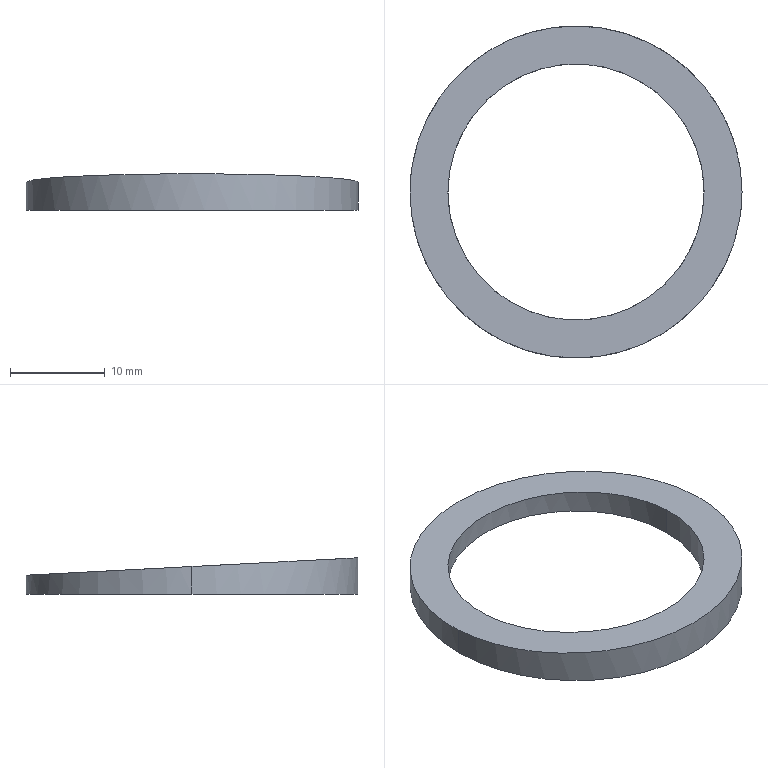Part | STEP file | TCHK-2D-D30-BB-5.stp.STEP | 1 solid | 6 faces | box 35 x 35 x 3.834 mm | volume 1137 mm3 | cylinder 4 | plane 2 | commonest cylinder face diameters 27 x2 35 x2
STEP:
#1=CARTESIAN_POINT('',(13.5,0.,0.));
#2=VERTEX_POINT('',#1);
#3=CARTESIAN_POINT('',(-13.5,0.,0.));
#4=VERTEX_POINT('',#3);
#5=CARTESIAN_POINT('',(0.,0.,0.));
#6=DIRECTION('',(0.,0.,-1.));
#7=DIRECTION('',(1.,0.,0.));
#8=AXIS2_PLACEMENT_3D('',#5,#6,#7);
#9=CIRCLE('',#8,13.5);
#10=EDGE_CURVE('',#2,#4,#9,.T.);
#11=ORIENTED_EDGE('',*,*,#10,.F.);
#12=CARTESIAN_POINT('',(0.,0.,0.));
#13=DIRECTION('',(0.,0.,-1.));
#14=DIRECTION('',(-1.,0.,0.));
#15=AXIS2_PLACEMENT_3D('',#12,#13,#14);
#16=CIRCLE('',#15,13.5);
#17=EDGE_CURVE('',#4,#2,#16,.T.);
#18=ORIENTED_EDGE('',*,*,#17,.F.);
#19=EDGE_LOOP('',(#11,#18));
#20=FACE_BOUND('',#19,.T.);
#21=CARTESIAN_POINT('',(-17.5,0.,0.));
#22=VERTEX_POINT('',#21);
#23=CARTESIAN_POINT('',(17.5,0.,0.));
#24=VERTEX_POINT('',#23);
#25=CARTESIAN_POINT('',(0.,0.,0.));
#26=DIRECTION('',(0.,0.,1.));
#27=DIRECTION('',(-1.,0.,0.));
#28=AXIS2_PLACEMENT_3D('',#25,#26,#27);
#29=CIRCLE('',#28,17.5);
#30=EDGE_CURVE('',#22,#24,#29,.T.);
#31=ORIENTED_EDGE('',*,*,#30,.F.);
#32=CARTESIAN_POINT('',(0.,0.,0.));
#33=DIRECTION('',(0.,0.,1.));
#34=DIRECTION('',(1.,0.,0.));
#35=AXIS2_PLACEMENT_3D('',#32,#33,#34);
#36=CIRCLE('',#35,17.5);
#37=EDGE_CURVE('',#24,#22,#36,.T.);
#38=ORIENTED_EDGE('',*,*,#37,.F.);
#39=EDGE_LOOP('',(#31,#38));
#40=FACE_OUTER_BOUND('',#39,.T.);
#41=CARTESIAN_POINT('',(0.,0.,0.));
#42=DIRECTION('',(0.,0.,1.));
#43=DIRECTION('',(1.,0.,0.));
#44=AXIS2_PLACEMENT_3D('',#41,#42,#43);
#45=PLANE('',#44);
#46=ADVANCED_FACE('',(#20,#40),#45,.F.);
#47=CARTESIAN_POINT('',(17.5,0.,2.917));
#48=VERTEX_POINT('',#47);
#49=CARTESIAN_POINT('',(17.5,0.,0.));
#50=DIRECTION('',(0.,0.,1.));
#51=VECTOR('',#50,1000.);
#52=LINE('',#49,#51);
#53=EDGE_CURVE('',#24,#48,#52,.T.);
#54=ORIENTED_EDGE('',*,*,#53,.F.);
#55=ORIENTED_EDGE('',*,*,#37,.T.);
#56=CARTESIAN_POINT('',(-17.5,0.,2.917));
#57=VERTEX_POINT('',#56);
#58=CARTESIAN_POINT('',(-17.5,0.,0.));
#59=DIRECTION('',(0.,0.,1.));
#60=VECTOR('',#59,1000.);
#61=LINE('',#58,#60);
#62=EDGE_CURVE('',#22,#57,#61,.T.);
#63=ORIENTED_EDGE('',*,*,#62,.T.);
#64=CARTESIAN_POINT('',(17.5,0.,2.917));
#65=CARTESIAN_POINT('',(17.5,0.5353,2.889));
#66=CARTESIAN_POINT('',(17.463,1.335,2.847));
#67=CARTESIAN_POINT('',(17.357,2.262,2.799));
#68=CARTESIAN_POINT('',(17.288,2.723,2.774));
#69=CARTESIAN_POINT('',(17.249,2.954,2.762));
#70=CARTESIAN_POINT('',(17.232,3.053,2.757));
#71=CARTESIAN_POINT('',(17.22,3.119,2.754));
#72=CARTESIAN_POINT('',(17.214,3.149,2.752));
#73=CARTESIAN_POINT('',(17.105,3.742,2.721));
#74=CARTESIAN_POINT('',(16.91,4.568,2.678));
#75=CARTESIAN_POINT('',(16.614,5.512,2.628));
#76=CARTESIAN_POINT('',(16.448,5.978,2.604));
#77=CARTESIAN_POINT('',(16.361,6.21,2.592));
#78=CARTESIAN_POINT('',(16.323,6.31,2.586));
#79=CARTESIAN_POINT('',(16.297,6.376,2.583));
#80=CARTESIAN_POINT('',(16.285,6.407,2.581));
#81=CARTESIAN_POINT('',(16.054,6.991,2.551));
#82=CARTESIAN_POINT('',(15.687,7.796,2.509));
#83=CARTESIAN_POINT('',(15.191,8.698,2.461));
#84=CARTESIAN_POINT('',(14.925,9.14,2.438));
#85=CARTESIAN_POINT('',(14.807,9.328,2.428));
#86=CARTESIAN_POINT('',(14.728,9.452,2.422));
#87=CARTESIAN_POINT('',(14.689,9.513,2.419));
#88=CARTESIAN_POINT('',(13.987,10.587,2.362));
#89=CARTESIAN_POINT('',(13.228,11.521,2.313));
#90=CARTESIAN_POINT('',(11.948,12.801,2.246));
#91=CARTESIAN_POINT('',(11.278,13.406,2.215));
#92=CARTESIAN_POINT('',(10.444,14.047,2.181));
#93=CARTESIAN_POINT('',(10.015,14.353,2.165));
#94=CARTESIAN_POINT('',(9.828,14.48,2.158));
#95=CARTESIAN_POINT('',(9.702,14.564,2.154));
#96=CARTESIAN_POINT('',(9.638,14.607,2.152));
#97=CARTESIAN_POINT('',(9.082,14.971,2.133));
#98=CARTESIAN_POINT('',(8.319,15.416,2.109));
#99=CARTESIAN_POINT('',(7.393,15.867,2.086));
#100=CARTESIAN_POINT('',(6.92,16.075,2.075));
#101=CARTESIAN_POINT('',(6.682,16.174,2.069));
#102=CARTESIAN_POINT('',(6.579,16.216,2.067));
#103=CARTESIAN_POINT('',(6.51,16.244,2.066));
#104=CARTESIAN_POINT('',(6.475,16.258,2.065));
#105=CARTESIAN_POINT('',(5.915,16.48,2.053));
#106=CARTESIAN_POINT('',(5.113,16.754,2.039));
#107=CARTESIAN_POINT('',(4.155,17.004,2.026));
#108=CARTESIAN_POINT('',(3.672,17.112,2.02));
#109=CARTESIAN_POINT('',(3.428,17.161,2.018));
#110=CARTESIAN_POINT('',(3.324,17.181,2.017));
#111=CARTESIAN_POINT('',(3.254,17.195,2.016));
#112=CARTESIAN_POINT('',(3.217,17.202,2.016));
#113=CARTESIAN_POINT('',(2.133,17.403,2.005));
#114=CARTESIAN_POINT('',(1.07,17.5,2.));
#115=CARTESIAN_POINT('',(-0.535,17.5,2.));
#116=CARTESIAN_POINT('',(-1.334,17.464,2.002));
#117=CARTESIAN_POINT('',(-2.261,17.357,2.007));
#118=CARTESIAN_POINT('',(-2.723,17.288,2.011));
#119=CARTESIAN_POINT('',(-2.954,17.249,2.013));
#120=CARTESIAN_POINT('',(-3.053,17.232,2.014));
#121=CARTESIAN_POINT('',(-3.119,17.22,2.015));
#122=CARTESIAN_POINT('',(-3.149,17.214,2.015));
#123=CARTESIAN_POINT('',(-3.743,17.105,2.021));
#124=CARTESIAN_POINT('',(-4.569,16.91,2.031));
#125=CARTESIAN_POINT('',(-5.512,16.614,2.046));
#126=CARTESIAN_POINT('',(-5.978,16.448,2.055));
#127=CARTESIAN_POINT('',(-6.21,16.361,2.06));
#128=CARTESIAN_POINT('',(-6.31,16.323,2.062));
#129=CARTESIAN_POINT('',(-6.376,16.297,2.063));
#130=CARTESIAN_POINT('',(-6.407,16.285,2.064));
#131=CARTESIAN_POINT('',(-6.992,16.054,2.076));
#132=CARTESIAN_POINT('',(-7.796,15.687,2.095));
#133=CARTESIAN_POINT('',(-8.698,15.19,2.121));
#134=CARTESIAN_POINT('',(-9.14,14.925,2.135));
#135=CARTESIAN_POINT('',(-9.328,14.807,2.141));
#136=CARTESIAN_POINT('',(-9.452,14.728,2.145));
#137=CARTESIAN_POINT('',(-9.513,14.689,2.147));
#138=CARTESIAN_POINT('',(-10.587,13.987,2.184));
#139=CARTESIAN_POINT('',(-11.521,13.228,2.224));
#140=CARTESIAN_POINT('',(-12.801,11.948,2.291));
#141=CARTESIAN_POINT('',(-13.405,11.278,2.326));
#142=CARTESIAN_POINT('',(-14.047,10.444,2.37));
#143=CARTESIAN_POINT('',(-14.353,10.015,2.392));
#144=CARTESIAN_POINT('',(-14.48,9.828,2.402));
#145=CARTESIAN_POINT('',(-14.564,9.702,2.409));
#146=CARTESIAN_POINT('',(-14.607,9.638,2.412));
#147=CARTESIAN_POINT('',(-14.971,9.082,2.441));
#148=CARTESIAN_POINT('',(-15.416,8.319,2.481));
#149=CARTESIAN_POINT('',(-15.867,7.393,2.53));
#150=CARTESIAN_POINT('',(-16.075,6.92,2.554));
#151=CARTESIAN_POINT('',(-16.174,6.682,2.567));
#152=CARTESIAN_POINT('',(-16.216,6.579,2.572));
#153=CARTESIAN_POINT('',(-16.244,6.51,2.576));
#154=CARTESIAN_POINT('',(-16.258,6.475,2.578));
#155=CARTESIAN_POINT('',(-16.48,5.915,2.607));
#156=CARTESIAN_POINT('',(-16.754,5.112,2.649));
#157=CARTESIAN_POINT('',(-17.004,4.155,2.699));
#158=CARTESIAN_POINT('',(-17.112,3.672,2.725));
#159=CARTESIAN_POINT('',(-17.161,3.428,2.737));
#160=CARTESIAN_POINT('',(-17.181,3.324,2.743));
#161=CARTESIAN_POINT('',(-17.195,3.254,2.747));
#162=CARTESIAN_POINT('',(-17.202,3.217,2.749));
#163=CARTESIAN_POINT('',(-17.403,2.133,2.805));
#164=CARTESIAN_POINT('',(-17.5,1.071,2.861));
#165=CARTESIAN_POINT('',(-17.5,0.,2.917));
#166=B_SPLINE_CURVE_WITH_KNOTS('',3,(#64,#65,#66,#67,#68,#69,#70,#71,#72,#73,#74,#75,#76,#77,#78,#79,#80,#81,#82,#83,#84,#85,#86,#87,#88,#89,#90,#91,#92,#93,#94,#95,#96,#97,#98,#99,#100,#101,#102,#103,#104,#105,#106,#107,#108,#109,#110,#111,#112,#113,#114,#115,#116,#117,#118,#119,#120,#121,#122,#123,#124,#125,#126,#127,#128,#129,#130,#131,#132,#133,#134,#135,#136,#137,#138,#139,#140,#141,#142,#143,#144,#145,#146,#147,#148,#149,#150,#151,#152,#153,#154,#155,#156,#157,#158,#159,#160,#161,#162,#163,#164,#165),.UNSPECIFIED.,.F.,.F.,(4,1,1,1,1,2,2,1,1,1,1,2,2,1,1,1,2,2,2,1,1,1,2,2,1,1,1,1,2,2,1,1,1,1,2,2,2,1,1,1,1,2,2,1,1,1,1,2,2,1,1,1,2,2,2,1,1,1,2,2,1,1,1,1,2,2,1,1,1,1,2,2,4),(0.,0.03125,0.04688,0.05469,0.05859,0.06055,0.0625,0.09375,0.1094,0.1172,0.1211,0.123,0.125,0.1562,0.1719,0.1797,0.1836,0.1875,0.25,0.2812,0.2969,0.3047,0.3086,0.3125,0.3437,0.3594,0.3672,0.3711,0.373,0.375,0.4062,0.4219,0.4297,0.4336,0.4355,0.4375,0.5,0.5312,0.5469,0.5547,0.5586,0.5605,0.5625,0.5937,0.6094,0.6172,0.6211,0.623,0.625,0.6562,0.6719,0.6797,0.6836,0.6875,0.75,0.7812,0.7969,0.8047,0.8086,0.8125,0.8437,0.8594,0.8672,0.8711,0.873,0.875,0.9062,0.9219,0.9297,0.9336,0.9355,0.9375,1.),.UNSPECIFIED.);
#167=EDGE_CURVE('',#48,#57,#166,.T.);
#168=ORIENTED_EDGE('',*,*,#167,.F.);
#169=EDGE_LOOP('',(#54,#55,#63,#168));
#170=FACE_OUTER_BOUND('',#169,.T.);
#171=CARTESIAN_POINT('',(0.,0.,0.));
#172=DIRECTION('',(0.,0.,1.));
#173=DIRECTION('',(1.,0.,0.));
#174=AXIS2_PLACEMENT_3D('',#171,#172,#173);
#175=CYLINDRICAL_SURFACE('',#174,17.5);
#176=ADVANCED_FACE('',(#170),#175,.T.);
#177=CARTESIAN_POINT('',(13.5,0.,2.917));
#178=VERTEX_POINT('',#177);
#179=CARTESIAN_POINT('',(-13.5,0.,2.917));
#180=VERTEX_POINT('',#179);
#181=CARTESIAN_POINT('',(13.5,0.,2.917));
#182=CARTESIAN_POINT('',(13.5,-0.4129,2.939));
#183=CARTESIAN_POINT('',(13.472,-1.03,2.971));
#184=CARTESIAN_POINT('',(13.39,-1.745,3.009));
#185=CARTESIAN_POINT('',(13.336,-2.101,3.027));
#186=CARTESIAN_POINT('',(13.306,-2.279,3.037));
#187=CARTESIAN_POINT('',(13.293,-2.355,3.041));
#188=CARTESIAN_POINT('',(13.284,-2.406,3.043));
#189=CARTESIAN_POINT('',(13.28,-2.43,3.044));
#190=CARTESIAN_POINT('',(13.195,-2.887,3.068));
#191=CARTESIAN_POINT('',(13.045,-3.524,3.102));
#192=CARTESIAN_POINT('',(12.816,-4.252,3.14));
#193=CARTESIAN_POINT('',(12.689,-4.612,3.159));
#194=CARTESIAN_POINT('',(12.622,-4.791,3.168));
#195=CARTESIAN_POINT('',(12.592,-4.867,3.172));
#196=CARTESIAN_POINT('',(12.572,-4.918,3.175));
#197=CARTESIAN_POINT('',(12.563,-4.943,3.176));
#198=CARTESIAN_POINT('',(12.384,-5.393,3.2));
#199=CARTESIAN_POINT('',(12.102,-6.014,3.232));
#200=CARTESIAN_POINT('',(11.719,-6.71,3.269));
#201=CARTESIAN_POINT('',(11.513,-7.051,3.287));
#202=CARTESIAN_POINT('',(11.423,-7.196,3.294));
#203=CARTESIAN_POINT('',(11.362,-7.292,3.299));
#204=CARTESIAN_POINT('',(11.331,-7.339,3.302));
#205=CARTESIAN_POINT('',(10.79,-8.167,3.345));
#206=CARTESIAN_POINT('',(10.204,-8.887,3.383));
#207=CARTESIAN_POINT('',(9.217,-9.875,3.435));
#208=CARTESIAN_POINT('',(8.7,-10.341,3.459));
#209=CARTESIAN_POINT('',(8.057,-10.837,3.485));
#210=CARTESIAN_POINT('',(7.726,-11.072,3.497));
#211=CARTESIAN_POINT('',(7.581,-11.17,3.503));
#212=CARTESIAN_POINT('',(7.485,-11.235,3.506));
#213=CARTESIAN_POINT('',(7.435,-11.268,3.508));
#214=CARTESIAN_POINT('',(7.006,-11.549,3.522));
#215=CARTESIAN_POINT('',(6.418,-11.892,3.54));
#216=CARTESIAN_POINT('',(5.703,-12.24,3.559));
#217=CARTESIAN_POINT('',(5.339,-12.4,3.567));
#218=CARTESIAN_POINT('',(5.155,-12.477,3.571));
#219=CARTESIAN_POINT('',(5.075,-12.51,3.573));
#220=CARTESIAN_POINT('',(5.022,-12.531,3.574));
#221=CARTESIAN_POINT('',(4.995,-12.542,3.574));
#222=CARTESIAN_POINT('',(4.563,-12.713,3.583));
#223=CARTESIAN_POINT('',(3.944,-12.924,3.594));
#224=CARTESIAN_POINT('',(3.205,-13.117,3.605));
#225=CARTESIAN_POINT('',(2.832,-13.2,3.609));
#226=CARTESIAN_POINT('',(2.645,-13.239,3.611));
#227=CARTESIAN_POINT('',(2.564,-13.254,3.612));
#228=CARTESIAN_POINT('',(2.51,-13.265,3.612));
#229=CARTESIAN_POINT('',(2.482,-13.27,3.613));
#230=CARTESIAN_POINT('',(1.645,-13.425,3.621));
#231=CARTESIAN_POINT('',(0.8248,-13.5,3.625));
#232=CARTESIAN_POINT('',(-0.4124,-13.5,3.625));
#233=CARTESIAN_POINT('',(-1.029,-13.472,3.623));
#234=CARTESIAN_POINT('',(-1.744,-13.39,3.619));
#235=CARTESIAN_POINT('',(-2.101,-13.336,3.616));
#236=CARTESIAN_POINT('',(-2.279,-13.306,3.614));
#237=CARTESIAN_POINT('',(-2.355,-13.293,3.614));
#238=CARTESIAN_POINT('',(-2.406,-13.284,3.613));
#239=CARTESIAN_POINT('',(-2.43,-13.28,3.613));
#240=CARTESIAN_POINT('',(-2.887,-13.195,3.609));
#241=CARTESIAN_POINT('',(-3.524,-13.045,3.601));
#242=CARTESIAN_POINT('',(-4.252,-12.816,3.589));
#243=CARTESIAN_POINT('',(-4.612,-12.689,3.582));
#244=CARTESIAN_POINT('',(-4.791,-12.622,3.579));
#245=CARTESIAN_POINT('',(-4.867,-12.592,3.577));
#246=CARTESIAN_POINT('',(-4.918,-12.572,3.576));
#247=CARTESIAN_POINT('',(-4.943,-12.563,3.576));
#248=CARTESIAN_POINT('',(-5.393,-12.384,3.566));
#249=CARTESIAN_POINT('',(-6.014,-12.102,3.551));
#250=CARTESIAN_POINT('',(-6.71,-11.718,3.531));
#251=CARTESIAN_POINT('',(-7.051,-11.513,3.521));
#252=CARTESIAN_POINT('',(-7.196,-11.423,3.516));
#253=CARTESIAN_POINT('',(-7.292,-11.362,3.513));
#254=CARTESIAN_POINT('',(-7.339,-11.331,3.511));
#255=CARTESIAN_POINT('',(-8.167,-10.79,3.483));
#256=CARTESIAN_POINT('',(-8.887,-10.204,3.452));
#257=CARTESIAN_POINT('',(-9.875,-9.217,3.4));
#258=CARTESIAN_POINT('',(-10.341,-8.7,3.373));
#259=CARTESIAN_POINT('',(-10.837,-8.057,3.339));
#260=CARTESIAN_POINT('',(-11.072,-7.726,3.322));
#261=CARTESIAN_POINT('',(-11.17,-7.581,3.314));
#262=CARTESIAN_POINT('',(-11.235,-7.485,3.309));
#263=CARTESIAN_POINT('',(-11.268,-7.435,3.307));
#264=CARTESIAN_POINT('',(-11.549,-7.006,3.284));
#265=CARTESIAN_POINT('',(-11.892,-6.418,3.253));
#266=CARTESIAN_POINT('',(-12.24,-5.703,3.216));
#267=CARTESIAN_POINT('',(-12.401,-5.338,3.197));
#268=CARTESIAN_POINT('',(-12.477,-5.154,3.187));
#269=CARTESIAN_POINT('',(-12.51,-5.075,3.183));
#270=CARTESIAN_POINT('',(-12.531,-5.022,3.18));
#271=CARTESIAN_POINT('',(-12.542,-4.995,3.179));
#272=CARTESIAN_POINT('',(-12.713,-4.563,3.156));
#273=CARTESIAN_POINT('',(-12.924,-3.944,3.124));
#274=CARTESIAN_POINT('',(-13.117,-3.206,3.085));
#275=CARTESIAN_POINT('',(-13.2,-2.832,3.066));
#276=CARTESIAN_POINT('',(-13.239,-2.645,3.056));
#277=CARTESIAN_POINT('',(-13.254,-2.564,3.052));
#278=CARTESIAN_POINT('',(-13.265,-2.51,3.049));
#279=CARTESIAN_POINT('',(-13.27,-2.482,3.047));
#280=CARTESIAN_POINT('',(-13.425,-1.645,3.003));
#281=CARTESIAN_POINT('',(-13.5,-0.8265,2.96));
#282=CARTESIAN_POINT('',(-13.5,0.,2.917));
#283=B_SPLINE_CURVE_WITH_KNOTS('',3,(#181,#182,#183,#184,#185,#186,#187,#188,#189,#190,#191,#192,#193,#194,#195,#196,#197,#198,#199,#200,#201,#202,#203,#204,#205,#206,#207,#208,#209,#210,#211,#212,#213,#214,#215,#216,#217,#218,#219,#220,#221,#222,#223,#224,#225,#226,#227,#228,#229,#230,#231,#232,#233,#234,#235,#236,#237,#238,#239,#240,#241,#242,#243,#244,#245,#246,#247,#248,#249,#250,#251,#252,#253,#254,#255,#256,#257,#258,#259,#260,#261,#262,#263,#264,#265,#266,#267,#268,#269,#270,#271,#272,#273,#274,#275,#276,#277,#278,#279,#280,#281,#282),.UNSPECIFIED.,.F.,.F.,(4,1,1,1,1,2,2,1,1,1,1,2,2,1,1,1,2,2,2,1,1,1,2,2,1,1,1,1,2,2,1,1,1,1,2,2,2,1,1,1,1,2,2,1,1,1,1,2,2,1,1,1,2,2,2,1,1,1,2,2,1,1,1,1,2,2,1,1,1,1,2,2,4),(0.,0.03125,0.04687,0.05469,0.05859,0.06055,0.0625,0.09375,0.1094,0.1172,0.1211,0.123,0.125,0.1562,0.1719,0.1797,0.1836,0.1875,0.25,0.2812,0.2969,0.3047,0.3086,0.3125,0.3437,0.3594,0.3672,0.3711,0.373,0.375,0.4062,0.4219,0.4297,0.4336,0.4355,0.4375,0.5,0.5312,0.5469,0.5547,0.5586,0.5605,0.5625,0.5937,0.6094,0.6172,0.6211,0.623,0.625,0.6562,0.6719,0.6797,0.6836,0.6875,0.75,0.7812,0.7969,0.8047,0.8086,0.8125,0.8437,0.8594,0.8672,0.8711,0.873,0.875,0.9062,0.9219,0.9297,0.9336,0.9355,0.9375,1.),.UNSPECIFIED.);
#284=EDGE_CURVE('',#178,#180,#283,.T.);
#285=ORIENTED_EDGE('',*,*,#284,.T.);
#286=CARTESIAN_POINT('',(-13.5,0.,2.917));
#287=CARTESIAN_POINT('',(-13.5,0.4129,2.895));
#288=CARTESIAN_POINT('',(-13.472,1.03,2.863));
#289=CARTESIAN_POINT('',(-13.39,1.745,2.826));
#290=CARTESIAN_POINT('',(-13.336,2.101,2.807));
#291=CARTESIAN_POINT('',(-13.306,2.279,2.798));
#292=CARTESIAN_POINT('',(-13.293,2.355,2.794));
#293=CARTESIAN_POINT('',(-13.284,2.406,2.791));
#294=CARTESIAN_POINT('',(-13.28,2.43,2.79));
#295=CARTESIAN_POINT('',(-13.195,2.887,2.766));
#296=CARTESIAN_POINT('',(-13.045,3.524,2.732));
#297=CARTESIAN_POINT('',(-12.816,4.252,2.694));
#298=CARTESIAN_POINT('',(-12.689,4.612,2.675));
#299=CARTESIAN_POINT('',(-12.622,4.791,2.666));
#300=CARTESIAN_POINT('',(-12.592,4.867,2.662));
#301=CARTESIAN_POINT('',(-12.572,4.918,2.659));
#302=CARTESIAN_POINT('',(-12.563,4.943,2.658));
#303=CARTESIAN_POINT('',(-12.384,5.393,2.634));
#304=CARTESIAN_POINT('',(-12.102,6.014,2.602));
#305=CARTESIAN_POINT('',(-11.719,6.71,2.565));
#306=CARTESIAN_POINT('',(-11.513,7.051,2.548));
#307=CARTESIAN_POINT('',(-11.423,7.196,2.54));
#308=CARTESIAN_POINT('',(-11.362,7.292,2.535));
#309=CARTESIAN_POINT('',(-11.331,7.339,2.533));
#310=CARTESIAN_POINT('',(-10.79,8.167,2.489));
#311=CARTESIAN_POINT('',(-10.204,8.887,2.451));
#312=CARTESIAN_POINT('',(-9.217,9.875,2.4));
#313=CARTESIAN_POINT('',(-8.7,10.341,2.375));
#314=CARTESIAN_POINT('',(-8.057,10.837,2.349));
#315=CARTESIAN_POINT('',(-7.726,11.072,2.337));
#316=CARTESIAN_POINT('',(-7.581,11.17,2.332));
#317=CARTESIAN_POINT('',(-7.485,11.235,2.328));
#318=CARTESIAN_POINT('',(-7.435,11.268,2.327));
#319=CARTESIAN_POINT('',(-7.006,11.549,2.312));
#320=CARTESIAN_POINT('',(-6.418,11.892,2.294));
#321=CARTESIAN_POINT('',(-5.703,12.24,2.276));
#322=CARTESIAN_POINT('',(-5.339,12.4,2.267));
#323=CARTESIAN_POINT('',(-5.155,12.477,2.263));
#324=CARTESIAN_POINT('',(-5.075,12.51,2.262));
#325=CARTESIAN_POINT('',(-5.022,12.531,2.26));
#326=CARTESIAN_POINT('',(-4.995,12.542,2.26));
#327=CARTESIAN_POINT('',(-4.563,12.713,2.251));
#328=CARTESIAN_POINT('',(-3.944,12.924,2.24));
#329=CARTESIAN_POINT('',(-3.205,13.117,2.23));
#330=CARTESIAN_POINT('',(-2.832,13.2,2.225));
#331=CARTESIAN_POINT('',(-2.645,13.239,2.223));
#332=CARTESIAN_POINT('',(-2.564,13.254,2.223));
#333=CARTESIAN_POINT('',(-2.51,13.265,2.222));
#334=CARTESIAN_POINT('',(-2.482,13.27,2.222));
#335=CARTESIAN_POINT('',(-1.645,13.425,2.214));
#336=CARTESIAN_POINT('',(-0.8248,13.5,2.21));
#337=CARTESIAN_POINT('',(0.4124,13.5,2.21));
#338=CARTESIAN_POINT('',(1.029,13.472,2.211));
#339=CARTESIAN_POINT('',(1.744,13.39,2.215));
#340=CARTESIAN_POINT('',(2.101,13.336,2.218));
#341=CARTESIAN_POINT('',(2.279,13.306,2.22));
#342=CARTESIAN_POINT('',(2.355,13.293,2.22));
#343=CARTESIAN_POINT('',(2.406,13.284,2.221));
#344=CARTESIAN_POINT('',(2.43,13.28,2.221));
#345=CARTESIAN_POINT('',(2.887,13.195,2.226));
#346=CARTESIAN_POINT('',(3.524,13.045,2.233));
#347=CARTESIAN_POINT('',(4.252,12.816,2.245));
#348=CARTESIAN_POINT('',(4.612,12.689,2.252));
#349=CARTESIAN_POINT('',(4.791,12.622,2.256));
#350=CARTESIAN_POINT('',(4.867,12.592,2.257));
#351=CARTESIAN_POINT('',(4.918,12.572,2.258));
#352=CARTESIAN_POINT('',(4.943,12.563,2.259));
#353=CARTESIAN_POINT('',(5.393,12.384,2.268));
#354=CARTESIAN_POINT('',(6.014,12.102,2.283));
#355=CARTESIAN_POINT('',(6.71,11.718,2.303));
#356=CARTESIAN_POINT('',(7.051,11.513,2.314));
#357=CARTESIAN_POINT('',(7.196,11.423,2.319));
#358=CARTESIAN_POINT('',(7.292,11.362,2.322));
#359=CARTESIAN_POINT('',(7.339,11.331,2.323));
#360=CARTESIAN_POINT('',(8.167,10.79,2.352));
#361=CARTESIAN_POINT('',(8.887,10.204,2.382));
#362=CARTESIAN_POINT('',(9.875,9.217,2.434));
#363=CARTESIAN_POINT('',(10.341,8.7,2.461));
#364=CARTESIAN_POINT('',(10.837,8.057,2.495));
#365=CARTESIAN_POINT('',(11.072,7.726,2.512));
#366=CARTESIAN_POINT('',(11.17,7.581,2.52));
#367=CARTESIAN_POINT('',(11.235,7.485,2.525));
#368=CARTESIAN_POINT('',(11.268,7.435,2.527));
#369=CARTESIAN_POINT('',(11.549,7.006,2.55));
#370=CARTESIAN_POINT('',(11.892,6.418,2.581));
#371=CARTESIAN_POINT('',(12.24,5.703,2.618));
#372=CARTESIAN_POINT('',(12.401,5.338,2.637));
#373=CARTESIAN_POINT('',(12.477,5.154,2.647));
#374=CARTESIAN_POINT('',(12.51,5.075,2.651));
#375=CARTESIAN_POINT('',(12.531,5.022,2.654));
#376=CARTESIAN_POINT('',(12.542,4.995,2.655));
#377=CARTESIAN_POINT('',(12.713,4.563,2.678));
#378=CARTESIAN_POINT('',(12.924,3.944,2.71));
#379=CARTESIAN_POINT('',(13.117,3.206,2.749));
#380=CARTESIAN_POINT('',(13.2,2.832,2.769));
#381=CARTESIAN_POINT('',(13.239,2.645,2.779));
#382=CARTESIAN_POINT('',(13.254,2.564,2.783));
#383=CARTESIAN_POINT('',(13.265,2.51,2.786));
#384=CARTESIAN_POINT('',(13.27,2.482,2.787));
#385=CARTESIAN_POINT('',(13.425,1.645,2.831));
#386=CARTESIAN_POINT('',(13.5,0.8265,2.874));
#387=CARTESIAN_POINT('',(13.5,0.,2.917));
#388=B_SPLINE_CURVE_WITH_KNOTS('',3,(#286,#287,#288,#289,#290,#291,#292,#293,#294,#295,#296,#297,#298,#299,#300,#301,#302,#303,#304,#305,#306,#307,#308,#309,#310,#311,#312,#313,#314,#315,#316,#317,#318,#319,#320,#321,#322,#323,#324,#325,#326,#327,#328,#329,#330,#331,#332,#333,#334,#335,#336,#337,#338,#339,#340,#341,#342,#343,#344,#345,#346,#347,#348,#349,#350,#351,#352,#353,#354,#355,#356,#357,#358,#359,#360,#361,#362,#363,#364,#365,#366,#367,#368,#369,#370,#371,#372,#373,#374,#375,#376,#377,#378,#379,#380,#381,#382,#383,#384,#385,#386,#387),.UNSPECIFIED.,.F.,.F.,(4,1,1,1,1,2,2,1,1,1,1,2,2,1,1,1,2,2,2,1,1,1,2,2,1,1,1,1,2,2,1,1,1,1,2,2,2,1,1,1,1,2,2,1,1,1,1,2,2,1,1,1,2,2,2,1,1,1,2,2,1,1,1,1,2,2,1,1,1,1,2,2,4),(0.,0.03125,0.04687,0.05469,0.05859,0.06055,0.0625,0.09375,0.1094,0.1172,0.1211,0.123,0.125,0.1562,0.1719,0.1797,0.1836,0.1875,0.25,0.2812,0.2969,0.3047,0.3086,0.3125,0.3437,0.3594,0.3672,0.3711,0.373,0.375,0.4063,0.4219,0.4297,0.4336,0.4355,0.4375,0.5,0.5312,0.5469,0.5547,0.5586,0.5605,0.5625,0.5937,0.6094,0.6172,0.6211,0.623,0.625,0.6562,0.6719,0.6797,0.6836,0.6875,0.75,0.7812,0.7969,0.8047,0.8086,0.8125,0.8437,0.8594,0.8672,0.8711,0.873,0.875,0.9062,0.9219,0.9297,0.9336,0.9355,0.9375,1.),.UNSPECIFIED.);
#389=EDGE_CURVE('',#180,#178,#388,.T.);
#390=ORIENTED_EDGE('',*,*,#389,.T.);
#391=EDGE_LOOP('',(#285,#390));
#392=FACE_BOUND('',#391,.T.);
#393=CARTESIAN_POINT('',(-17.5,0.,2.917));
#394=CARTESIAN_POINT('',(-17.5,-0.5353,2.945));
#395=CARTESIAN_POINT('',(-17.463,-1.335,2.987));
#396=CARTESIAN_POINT('',(-17.357,-2.262,3.036));
#397=CARTESIAN_POINT('',(-17.288,-2.723,3.06));
#398=CARTESIAN_POINT('',(-17.249,-2.954,3.072));
#399=CARTESIAN_POINT('',(-17.232,-3.053,3.077));
#400=CARTESIAN_POINT('',(-17.22,-3.119,3.081));
#401=CARTESIAN_POINT('',(-17.214,-3.149,3.082));
#402=CARTESIAN_POINT('',(-17.105,-3.742,3.113));
#403=CARTESIAN_POINT('',(-16.91,-4.568,3.157));
#404=CARTESIAN_POINT('',(-16.614,-5.512,3.206));
#405=CARTESIAN_POINT('',(-16.448,-5.978,3.23));
#406=CARTESIAN_POINT('',(-16.361,-6.21,3.243));
#407=CARTESIAN_POINT('',(-16.323,-6.31,3.248));
#408=CARTESIAN_POINT('',(-16.297,-6.376,3.251));
#409=CARTESIAN_POINT('',(-16.285,-6.407,3.253));
#410=CARTESIAN_POINT('',(-16.054,-6.991,3.284));
#411=CARTESIAN_POINT('',(-15.687,-7.796,3.326));
#412=CARTESIAN_POINT('',(-15.191,-8.698,3.373));
#413=CARTESIAN_POINT('',(-14.925,-9.14,3.396));
#414=CARTESIAN_POINT('',(-14.807,-9.328,3.406));
#415=CARTESIAN_POINT('',(-14.728,-9.452,3.413));
#416=CARTESIAN_POINT('',(-14.689,-9.513,3.416));
#417=CARTESIAN_POINT('',(-13.987,-10.587,3.472));
#418=CARTESIAN_POINT('',(-13.228,-11.521,3.521));
#419=CARTESIAN_POINT('',(-11.948,-12.801,3.588));
#420=CARTESIAN_POINT('',(-11.278,-13.406,3.62));
#421=CARTESIAN_POINT('',(-10.444,-14.047,3.653));
#422=CARTESIAN_POINT('',(-10.015,-14.353,3.669));
#423=CARTESIAN_POINT('',(-9.828,-14.48,3.676));
#424=CARTESIAN_POINT('',(-9.702,-14.564,3.68));
#425=CARTESIAN_POINT('',(-9.638,-14.607,3.683));
#426=CARTESIAN_POINT('',(-9.082,-14.971,3.702));
#427=CARTESIAN_POINT('',(-8.319,-15.416,3.725));
#428=CARTESIAN_POINT('',(-7.393,-15.867,3.749));
#429=CARTESIAN_POINT('',(-6.92,-16.075,3.76));
#430=CARTESIAN_POINT('',(-6.682,-16.174,3.765));
#431=CARTESIAN_POINT('',(-6.579,-16.216,3.767));
#432=CARTESIAN_POINT('',(-6.51,-16.244,3.768));
#433=CARTESIAN_POINT('',(-6.475,-16.258,3.769));
#434=CARTESIAN_POINT('',(-5.915,-16.48,3.781));
#435=CARTESIAN_POINT('',(-5.113,-16.754,3.795));
#436=CARTESIAN_POINT('',(-4.155,-17.004,3.808));
#437=CARTESIAN_POINT('',(-3.672,-17.112,3.814));
#438=CARTESIAN_POINT('',(-3.428,-17.161,3.817));
#439=CARTESIAN_POINT('',(-3.324,-17.181,3.818));
#440=CARTESIAN_POINT('',(-3.254,-17.195,3.818));
#441=CARTESIAN_POINT('',(-3.217,-17.202,3.819));
#442=CARTESIAN_POINT('',(-2.133,-17.403,3.829));
#443=CARTESIAN_POINT('',(-1.07,-17.5,3.834));
#444=CARTESIAN_POINT('',(0.535,-17.5,3.834));
#445=CARTESIAN_POINT('',(1.334,-17.464,3.832));
#446=CARTESIAN_POINT('',(2.261,-17.357,3.827));
#447=CARTESIAN_POINT('',(2.723,-17.288,3.823));
#448=CARTESIAN_POINT('',(2.954,-17.249,3.821));
#449=CARTESIAN_POINT('',(3.053,-17.232,3.82));
#450=CARTESIAN_POINT('',(3.119,-17.22,3.82));
#451=CARTESIAN_POINT('',(3.149,-17.214,3.819));
#452=CARTESIAN_POINT('',(3.743,-17.105,3.814));
#453=CARTESIAN_POINT('',(4.569,-16.91,3.803));
#454=CARTESIAN_POINT('',(5.512,-16.614,3.788));
#455=CARTESIAN_POINT('',(5.978,-16.448,3.779));
#456=CARTESIAN_POINT('',(6.21,-16.361,3.775));
#457=CARTESIAN_POINT('',(6.31,-16.323,3.773));
#458=CARTESIAN_POINT('',(6.376,-16.297,3.771));
#459=CARTESIAN_POINT('',(6.407,-16.285,3.771));
#460=CARTESIAN_POINT('',(6.992,-16.054,3.758));
#461=CARTESIAN_POINT('',(7.796,-15.687,3.739));
#462=CARTESIAN_POINT('',(8.698,-15.19,3.713));
#463=CARTESIAN_POINT('',(9.14,-14.925,3.699));
#464=CARTESIAN_POINT('',(9.328,-14.807,3.693));
#465=CARTESIAN_POINT('',(9.452,-14.728,3.689));
#466=CARTESIAN_POINT('',(9.513,-14.689,3.687));
#467=CARTESIAN_POINT('',(10.587,-13.987,3.65));
#468=CARTESIAN_POINT('',(11.521,-13.228,3.61));
#469=CARTESIAN_POINT('',(12.801,-11.948,3.543));
#470=CARTESIAN_POINT('',(13.405,-11.278,3.508));
#471=CARTESIAN_POINT('',(14.047,-10.444,3.464));
#472=CARTESIAN_POINT('',(14.353,-10.015,3.442));
#473=CARTESIAN_POINT('',(14.48,-9.828,3.432));
#474=CARTESIAN_POINT('',(14.564,-9.702,3.426));
#475=CARTESIAN_POINT('',(14.607,-9.638,3.422));
#476=CARTESIAN_POINT('',(14.971,-9.082,3.393));
#477=CARTESIAN_POINT('',(15.416,-8.319,3.353));
#478=CARTESIAN_POINT('',(15.867,-7.393,3.305));
#479=CARTESIAN_POINT('',(16.075,-6.92,3.28));
#480=CARTESIAN_POINT('',(16.174,-6.682,3.267));
#481=CARTESIAN_POINT('',(16.216,-6.579,3.262));
#482=CARTESIAN_POINT('',(16.244,-6.51,3.258));
#483=CARTESIAN_POINT('',(16.258,-6.475,3.256));
#484=CARTESIAN_POINT('',(16.48,-5.915,3.227));
#485=CARTESIAN_POINT('',(16.754,-5.112,3.185));
#486=CARTESIAN_POINT('',(17.004,-4.155,3.135));
#487=CARTESIAN_POINT('',(17.112,-3.672,3.11));
#488=CARTESIAN_POINT('',(17.161,-3.428,3.097));
#489=CARTESIAN_POINT('',(17.181,-3.324,3.091));
#490=CARTESIAN_POINT('',(17.195,-3.254,3.088));
#491=CARTESIAN_POINT('',(17.202,-3.217,3.086));
#492=CARTESIAN_POINT('',(17.403,-2.133,3.029));
#493=CARTESIAN_POINT('',(17.5,-1.071,2.973));
#494=CARTESIAN_POINT('',(17.5,0.,2.917));
#495=B_SPLINE_CURVE_WITH_KNOTS('',3,(#393,#394,#395,#396,#397,#398,#399,#400,#401,#402,#403,#404,#405,#406,#407,#408,#409,#410,#411,#412,#413,#414,#415,#416,#417,#418,#419,#420,#421,#422,#423,#424,#425,#426,#427,#428,#429,#430,#431,#432,#433,#434,#435,#436,#437,#438,#439,#440,#441,#442,#443,#444,#445,#446,#447,#448,#449,#450,#451,#452,#453,#454,#455,#456,#457,#458,#459,#460,#461,#462,#463,#464,#465,#466,#467,#468,#469,#470,#471,#472,#473,#474,#475,#476,#477,#478,#479,#480,#481,#482,#483,#484,#485,#486,#487,#488,#489,#490,#491,#492,#493,#494),.UNSPECIFIED.,.F.,.F.,(4,1,1,1,1,2,2,1,1,1,1,2,2,1,1,1,2,2,2,1,1,1,2,2,1,1,1,1,2,2,1,1,1,1,2,2,2,1,1,1,1,2,2,1,1,1,1,2,2,1,1,1,2,2,2,1,1,1,2,2,1,1,1,1,2,2,1,1,1,1,2,2,4),(0.,0.03125,0.04687,0.05469,0.05859,0.06055,0.0625,0.09375,0.1094,0.1172,0.1211,0.123,0.125,0.1562,0.1719,0.1797,0.1836,0.1875,0.25,0.2812,0.2969,0.3047,0.3086,0.3125,0.3437,0.3594,0.3672,0.3711,0.373,0.375,0.4062,0.4219,0.4297,0.4336,0.4355,0.4375,0.5,0.5312,0.5469,0.5547,0.5586,0.5605,0.5625,0.5937,0.6094,0.6172,0.6211,0.623,0.625,0.6562,0.6719,0.6797,0.6836,0.6875,0.75,0.7812,0.7969,0.8047,0.8086,0.8125,0.8437,0.8594,0.8672,0.8711,0.873,0.875,0.9062,0.9219,0.9297,0.9336,0.9355,0.9375,1.),.UNSPECIFIED.);
#496=EDGE_CURVE('',#57,#48,#495,.T.);
#497=ORIENTED_EDGE('',*,*,#496,.T.);
#498=ORIENTED_EDGE('',*,*,#167,.T.);
#499=EDGE_LOOP('',(#497,#498));
#500=FACE_OUTER_BOUND('',#499,.T.);
#501=CARTESIAN_POINT('',(50.,-17.5,3.834));
#502=DIRECTION('',(0.,-0.05234,-0.9986));
#503=DIRECTION('',(0.,-0.9986,0.05234));
#504=AXIS2_PLACEMENT_3D('',#501,#502,#503);
#505=PLANE('',#504);
#506=ADVANCED_FACE('',(#392,#500),#505,.F.);
#507=ORIENTED_EDGE('',*,*,#62,.F.);
#508=ORIENTED_EDGE('',*,*,#30,.T.);
#509=ORIENTED_EDGE('',*,*,#53,.T.);
#510=ORIENTED_EDGE('',*,*,#496,.F.);
#511=EDGE_LOOP('',(#507,#508,#509,#510));
#512=FACE_OUTER_BOUND('',#511,.T.);
#513=CARTESIAN_POINT('',(0.,0.,0.));
#514=DIRECTION('',(0.,0.,1.));
#515=DIRECTION('',(1.,0.,0.));
#516=AXIS2_PLACEMENT_3D('',#513,#514,#515);
#517=CYLINDRICAL_SURFACE('',#516,17.5);
#518=ADVANCED_FACE('',(#512),#517,.T.);
#519=CARTESIAN_POINT('',(13.5,0.,0.));
#520=DIRECTION('',(0.,0.,1.));
#521=VECTOR('',#520,1000.);
#522=LINE('',#519,#521);
#523=EDGE_CURVE('',#2,#178,#522,.T.);
#524=ORIENTED_EDGE('',*,*,#523,.T.);
#525=ORIENTED_EDGE('',*,*,#389,.F.);
#526=CARTESIAN_POINT('',(-13.5,0.,0.));
#527=DIRECTION('',(0.,0.,1.));
#528=VECTOR('',#527,1000.);
#529=LINE('',#526,#528);
#530=EDGE_CURVE('',#4,#180,#529,.T.);
#531=ORIENTED_EDGE('',*,*,#530,.F.);
#532=ORIENTED_EDGE('',*,*,#17,.T.);
#533=EDGE_LOOP('',(#524,#525,#531,#532));
#534=FACE_OUTER_BOUND('',#533,.T.);
#535=CARTESIAN_POINT('',(0.,0.,0.));
#536=DIRECTION('',(0.,0.,-1.));
#537=DIRECTION('',(-1.,0.,0.));
#538=AXIS2_PLACEMENT_3D('',#535,#536,#537);
#539=CYLINDRICAL_SURFACE('',#538,13.5);
#540=ADVANCED_FACE('',(#534),#539,.F.);
#541=ORIENTED_EDGE('',*,*,#530,.T.);
#542=ORIENTED_EDGE('',*,*,#284,.F.);
#543=ORIENTED_EDGE('',*,*,#523,.F.);
#544=ORIENTED_EDGE('',*,*,#10,.T.);
#545=EDGE_LOOP('',(#541,#542,#543,#544));
#546=FACE_OUTER_BOUND('',#545,.T.);
#547=CARTESIAN_POINT('',(0.,0.,0.));
#548=DIRECTION('',(0.,0.,-1.));
#549=DIRECTION('',(-1.,0.,0.));
#550=AXIS2_PLACEMENT_3D('',#547,#548,#549);
#551=CYLINDRICAL_SURFACE('',#550,13.5);
#552=ADVANCED_FACE('',(#546),#551,.F.);
#553=CLOSED_SHELL('',(#46,#176,#506,#518,#540,#552));
#554=MANIFOLD_SOLID_BREP('',#553);
#555=CARTESIAN_POINT('',(0.,0.,0.));
#556=DIRECTION('',(0.,0.,1.));
#557=DIRECTION('',(1.,0.,0.));
#558=AXIS2_PLACEMENT_3D('',#555,#556,#557);
#559=(LENGTH_UNIT()NAMED_UNIT(*)SI_UNIT(.MILLI.,.METRE.));
#560=UNCERTAINTY_MEASURE_WITH_UNIT(LENGTH_MEASURE(0.00001),#559,'','');
#561=(NAMED_UNIT(*)PLANE_ANGLE_UNIT()SI_UNIT($,.RADIAN.));
#562=(NAMED_UNIT(*)SI_UNIT($,.STERADIAN.)SOLID_ANGLE_UNIT());
#563=(GEOMETRIC_REPRESENTATION_CONTEXT(3)GLOBAL_UNCERTAINTY_ASSIGNED_CONTEXT((#560))GLOBAL_UNIT_ASSIGNED_CONTEXT((#559,#561,#562))REPRESENTATION_CONTEXT('',''));
#564=ADVANCED_BREP_SHAPE_REPRESENTATION('',(#554,#558),#563);